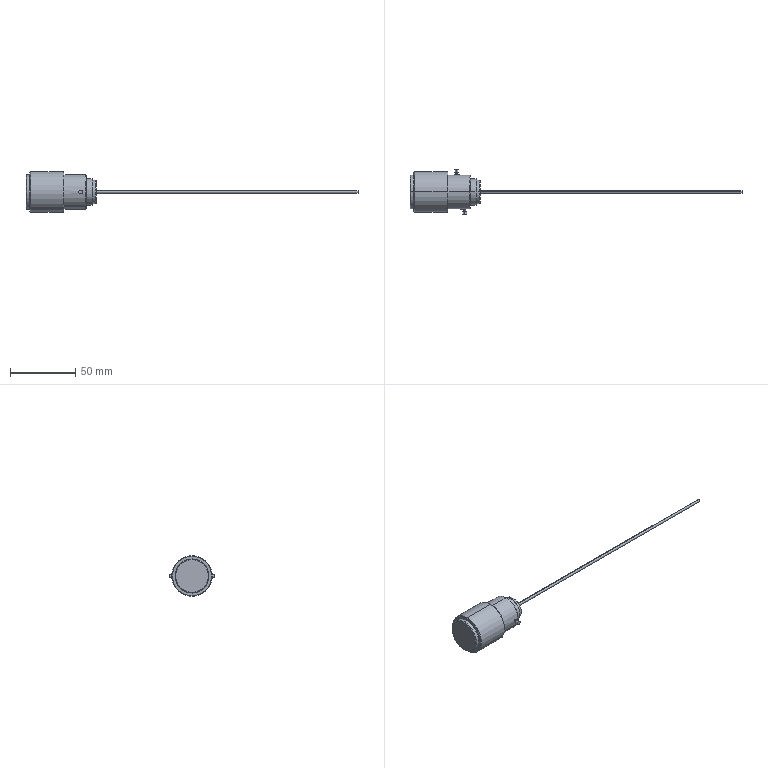Part | STEP file | Lens | 1 solid | 43 faces | box 253.5 x 35 x 31 mm | volume 33056 mm3 | cylinder 20 | cone 12 | plane 11 | commonest cylinder face diameters 26 x4 1.068 x2 1.193 x2 2 x2 2.761 x2 3 x2
STEP:
#1=CARTESIAN_POINT('',(-7.5,0.,-12.5));
#2=VERTEX_POINT('',#1);
#3=CARTESIAN_POINT('',(-7.5,0.,12.5));
#4=VERTEX_POINT('',#3);
#5=CARTESIAN_POINT('',(-7.5,0.,0.));
#6=DIRECTION('',(1.,0.,0.));
#7=DIRECTION('',(0.,0.,-1.));
#8=AXIS2_PLACEMENT_3D('',#5,#6,#7);
#9=CIRCLE('',#8,12.5);
#10=EDGE_CURVE('',#2,#4,#9,.T.);
#11=ORIENTED_EDGE('',*,*,#10,.F.);
#12=CARTESIAN_POINT('',(-8.,0.,-13.));
#13=VERTEX_POINT('',#12);
#14=CARTESIAN_POINT('',(-7.5,0.,-12.5));
#15=DIRECTION('',(-0.7071,0.,-0.7071));
#16=VECTOR('',#15,1000.);
#17=LINE('',#14,#16);
#18=EDGE_CURVE('',#2,#13,#17,.T.);
#19=ORIENTED_EDGE('',*,*,#18,.T.);
#20=CARTESIAN_POINT('',(-8.,0.,13.));
#21=VERTEX_POINT('',#20);
#22=CARTESIAN_POINT('',(-8.,0.,0.));
#23=DIRECTION('',(-1.,0.,0.));
#24=DIRECTION('',(0.,0.,-1.));
#25=AXIS2_PLACEMENT_3D('',#22,#23,#24);
#26=CIRCLE('',#25,13.);
#27=EDGE_CURVE('',#21,#13,#26,.T.);
#28=ORIENTED_EDGE('',*,*,#27,.F.);
#29=CARTESIAN_POINT('',(-7.5,0.,12.5));
#30=DIRECTION('',(-0.7071,0.,0.7071));
#31=VECTOR('',#30,1000.);
#32=LINE('',#29,#31);
#33=EDGE_CURVE('',#4,#21,#32,.T.);
#34=ORIENTED_EDGE('',*,*,#33,.F.);
#35=EDGE_LOOP('',(#11,#19,#28,#34));
#36=FACE_OUTER_BOUND('',#35,.T.);
#37=CARTESIAN_POINT('',(-7.5,0.,0.));
#38=DIRECTION('',(-1.,0.,0.));
#39=DIRECTION('',(0.,0.,1.));
#40=AXIS2_PLACEMENT_3D('',#37,#38,#39);
#41=CONICAL_SURFACE('',#40,12.5,0.7854);
#42=ADVANCED_FACE('',(#36),#41,.T.);
#43=CARTESIAN_POINT('',(0.,0.,-8.5));
#44=VERTEX_POINT('',#43);
#45=CARTESIAN_POINT('',(0.,0.,8.5));
#46=VERTEX_POINT('',#45);
#47=CARTESIAN_POINT('',(0.,0.,0.));
#48=DIRECTION('',(1.,0.,0.));
#49=DIRECTION('',(0.,0.,-1.));
#50=AXIS2_PLACEMENT_3D('',#47,#48,#49);
#51=CIRCLE('',#50,8.5);
#52=EDGE_CURVE('',#44,#46,#51,.T.);
#53=ORIENTED_EDGE('',*,*,#52,.F.);
#54=CARTESIAN_POINT('',(-0.5,0.,-9.));
#55=VERTEX_POINT('',#54);
#56=CARTESIAN_POINT('',(0.,0.,-8.5));
#57=DIRECTION('',(-0.7071,0.,-0.7071));
#58=VECTOR('',#57,1000.);
#59=LINE('',#56,#58);
#60=EDGE_CURVE('',#44,#55,#59,.T.);
#61=ORIENTED_EDGE('',*,*,#60,.T.);
#62=CARTESIAN_POINT('',(-0.5,0.,9.));
#63=VERTEX_POINT('',#62);
#64=CARTESIAN_POINT('',(-0.5,0.,0.));
#65=DIRECTION('',(-1.,0.,0.));
#66=DIRECTION('',(0.,0.,-1.));
#67=AXIS2_PLACEMENT_3D('',#64,#65,#66);
#68=CIRCLE('',#67,9.);
#69=EDGE_CURVE('',#63,#55,#68,.T.);
#70=ORIENTED_EDGE('',*,*,#69,.F.);
#71=CARTESIAN_POINT('',(0.,0.,8.5));
#72=DIRECTION('',(-0.7071,0.,0.7071));
#73=VECTOR('',#72,1000.);
#74=LINE('',#71,#73);
#75=EDGE_CURVE('',#46,#63,#74,.T.);
#76=ORIENTED_EDGE('',*,*,#75,.F.);
#77=EDGE_LOOP('',(#53,#61,#70,#76));
#78=FACE_OUTER_BOUND('',#77,.T.);
#79=CARTESIAN_POINT('',(0.,0.,0.));
#80=DIRECTION('',(-1.,0.,0.));
#81=DIRECTION('',(0.,0.,1.));
#82=AXIS2_PLACEMENT_3D('',#79,#80,#81);
#83=CONICAL_SURFACE('',#82,8.5,0.7854);
#84=ADVANCED_FACE('',(#78),#83,.T.);
#85=CARTESIAN_POINT('',(-2.5,0.,-9.5));
#86=VERTEX_POINT('',#85);
#87=CARTESIAN_POINT('',(-2.5,0.,9.5));
#88=VERTEX_POINT('',#87);
#89=CARTESIAN_POINT('',(-2.5,0.,0.));
#90=DIRECTION('',(1.,0.,0.));
#91=DIRECTION('',(0.,0.,-1.));
#92=AXIS2_PLACEMENT_3D('',#89,#90,#91);
#93=CIRCLE('',#92,9.5);
#94=EDGE_CURVE('',#86,#88,#93,.T.);
#95=ORIENTED_EDGE('',*,*,#94,.F.);
#96=CARTESIAN_POINT('',(-3.,0.,-10.));
#97=VERTEX_POINT('',#96);
#98=CARTESIAN_POINT('',(-2.5,0.,-9.5));
#99=DIRECTION('',(-0.7071,0.,-0.7071));
#100=VECTOR('',#99,1000.);
#101=LINE('',#98,#100);
#102=EDGE_CURVE('',#86,#97,#101,.T.);
#103=ORIENTED_EDGE('',*,*,#102,.T.);
#104=CARTESIAN_POINT('',(-3.,0.,10.));
#105=VERTEX_POINT('',#104);
#106=CARTESIAN_POINT('',(-3.,0.,0.));
#107=DIRECTION('',(-1.,0.,0.));
#108=DIRECTION('',(0.,0.,-1.));
#109=AXIS2_PLACEMENT_3D('',#106,#107,#108);
#110=CIRCLE('',#109,10.);
#111=EDGE_CURVE('',#105,#97,#110,.T.);
#112=ORIENTED_EDGE('',*,*,#111,.F.);
#113=CARTESIAN_POINT('',(-2.5,0.,9.5));
#114=DIRECTION('',(-0.7071,0.,0.7071));
#115=VECTOR('',#114,1000.);
#116=LINE('',#113,#115);
#117=EDGE_CURVE('',#88,#105,#116,.T.);
#118=ORIENTED_EDGE('',*,*,#117,.F.);
#119=EDGE_LOOP('',(#95,#103,#112,#118));
#120=FACE_OUTER_BOUND('',#119,.T.);
#121=CARTESIAN_POINT('',(-2.5,0.,0.));
#122=DIRECTION('',(-1.,0.,0.));
#123=DIRECTION('',(0.,0.,1.));
#124=AXIS2_PLACEMENT_3D('',#121,#122,#123);
#125=CONICAL_SURFACE('',#124,9.5,0.7854);
#126=ADVANCED_FACE('',(#120),#125,.T.);
#127=CARTESIAN_POINT('',(-24.5,0.,-15.));
#128=VERTEX_POINT('',#127);
#129=CARTESIAN_POINT('',(-24.5,0.,15.));
#130=VERTEX_POINT('',#129);
#131=CARTESIAN_POINT('',(-24.5,0.,0.));
#132=DIRECTION('',(1.,0.,0.));
#133=DIRECTION('',(0.,0.,-1.));
#134=AXIS2_PLACEMENT_3D('',#131,#132,#133);
#135=CIRCLE('',#134,15.);
#136=EDGE_CURVE('',#128,#130,#135,.T.);
#137=ORIENTED_EDGE('',*,*,#136,.F.);
#138=CARTESIAN_POINT('',(-25.,0.,-15.5));
#139=VERTEX_POINT('',#138);
#140=CARTESIAN_POINT('',(-24.5,0.,-15.));
#141=DIRECTION('',(-0.7071,0.,-0.7071));
#142=VECTOR('',#141,1000.);
#143=LINE('',#140,#142);
#144=EDGE_CURVE('',#128,#139,#143,.T.);
#145=ORIENTED_EDGE('',*,*,#144,.T.);
#146=CARTESIAN_POINT('',(-25.,0.,15.5));
#147=VERTEX_POINT('',#146);
#148=CARTESIAN_POINT('',(-25.,0.,0.));
#149=DIRECTION('',(-1.,0.,0.));
#150=DIRECTION('',(0.,0.,-1.));
#151=AXIS2_PLACEMENT_3D('',#148,#149,#150);
#152=CIRCLE('',#151,15.5);
#153=EDGE_CURVE('',#147,#139,#152,.T.);
#154=ORIENTED_EDGE('',*,*,#153,.F.);
#155=CARTESIAN_POINT('',(-24.5,0.,15.));
#156=DIRECTION('',(-0.7071,0.,0.7071));
#157=VECTOR('',#156,1000.);
#158=LINE('',#155,#157);
#159=EDGE_CURVE('',#130,#147,#158,.T.);
#160=ORIENTED_EDGE('',*,*,#159,.F.);
#161=EDGE_LOOP('',(#137,#145,#154,#160));
#162=FACE_OUTER_BOUND('',#161,.T.);
#163=CARTESIAN_POINT('',(-24.5,0.,0.));
#164=DIRECTION('',(-1.,0.,0.));
#165=DIRECTION('',(0.,0.,1.));
#166=AXIS2_PLACEMENT_3D('',#163,#164,#165);
#167=CONICAL_SURFACE('',#166,15.,0.7854);
#168=ADVANCED_FACE('',(#162),#167,.T.);
#169=CARTESIAN_POINT('',(-50.5,0.,15.));
#170=VERTEX_POINT('',#169);
#171=CARTESIAN_POINT('',(-50.5,0.,-15.));
#172=VERTEX_POINT('',#171);
#173=CARTESIAN_POINT('',(-50.5,0.,0.));
#174=DIRECTION('',(-1.,0.,0.));
#175=DIRECTION('',(0.,0.,1.));
#176=AXIS2_PLACEMENT_3D('',#173,#174,#175);
#177=CIRCLE('',#176,15.);
#178=EDGE_CURVE('',#170,#172,#177,.T.);
#179=ORIENTED_EDGE('',*,*,#178,.F.);
#180=CARTESIAN_POINT('',(-50.,0.,15.5));
#181=VERTEX_POINT('',#180);
#182=CARTESIAN_POINT('',(-50.,0.,15.5));
#183=DIRECTION('',(0.7071,0.,0.7071));
#184=VECTOR('',#183,1000.);
#185=LINE('',#182,#184);
#186=EDGE_CURVE('',#170,#181,#185,.T.);
#187=ORIENTED_EDGE('',*,*,#186,.T.);
#188=CARTESIAN_POINT('',(-50.,0.,-15.5));
#189=VERTEX_POINT('',#188);
#190=CARTESIAN_POINT('',(-50.,0.,0.));
#191=DIRECTION('',(1.,0.,0.));
#192=DIRECTION('',(0.,0.,1.));
#193=AXIS2_PLACEMENT_3D('',#190,#191,#192);
#194=CIRCLE('',#193,15.5);
#195=EDGE_CURVE('',#189,#181,#194,.T.);
#196=ORIENTED_EDGE('',*,*,#195,.F.);
#197=CARTESIAN_POINT('',(-50.,0.,-15.5));
#198=DIRECTION('',(0.7071,0.,-0.7071));
#199=VECTOR('',#198,1000.);
#200=LINE('',#197,#199);
#201=EDGE_CURVE('',#172,#189,#200,.T.);
#202=ORIENTED_EDGE('',*,*,#201,.F.);
#203=EDGE_LOOP('',(#179,#187,#196,#202));
#204=FACE_OUTER_BOUND('',#203,.T.);
#205=CARTESIAN_POINT('',(-50.,0.,0.));
#206=DIRECTION('',(1.,0.,0.));
#207=DIRECTION('',(0.,0.,-1.));
#208=AXIS2_PLACEMENT_3D('',#205,#206,#207);
#209=CONICAL_SURFACE('',#208,15.5,0.7854);
#210=ADVANCED_FACE('',(#204),#209,.T.);
#211=CARTESIAN_POINT('',(-53.5,0.,12.5));
#212=VERTEX_POINT('',#211);
#213=CARTESIAN_POINT('',(-53.5,0.,-12.5));
#214=VERTEX_POINT('',#213);
#215=CARTESIAN_POINT('',(-53.5,0.,0.));
#216=DIRECTION('',(-1.,0.,0.));
#217=DIRECTION('',(0.,0.,1.));
#218=AXIS2_PLACEMENT_3D('',#215,#216,#217);
#219=CIRCLE('',#218,12.5);
#220=EDGE_CURVE('',#212,#214,#219,.T.);
#221=ORIENTED_EDGE('',*,*,#220,.F.);
#222=CARTESIAN_POINT('',(-53.,0.,13.));
#223=VERTEX_POINT('',#222);
#224=CARTESIAN_POINT('',(-53.5,0.,12.5));
#225=DIRECTION('',(0.7071,0.,0.7071));
#226=VECTOR('',#225,1000.);
#227=LINE('',#224,#226);
#228=EDGE_CURVE('',#212,#223,#227,.T.);
#229=ORIENTED_EDGE('',*,*,#228,.T.);
#230=CARTESIAN_POINT('',(-53.,0.,-13.));
#231=VERTEX_POINT('',#230);
#232=CARTESIAN_POINT('',(-53.,0.,0.));
#233=DIRECTION('',(1.,0.,0.));
#234=DIRECTION('',(0.,0.,1.));
#235=AXIS2_PLACEMENT_3D('',#232,#233,#234);
#236=CIRCLE('',#235,13.);
#237=EDGE_CURVE('',#231,#223,#236,.T.);
#238=ORIENTED_EDGE('',*,*,#237,.F.);
#239=CARTESIAN_POINT('',(-53.5,0.,-12.5));
#240=DIRECTION('',(0.7071,0.,-0.7071));
#241=VECTOR('',#240,1000.);
#242=LINE('',#239,#241);
#243=EDGE_CURVE('',#214,#231,#242,.T.);
#244=ORIENTED_EDGE('',*,*,#243,.F.);
#245=EDGE_LOOP('',(#221,#229,#238,#244));
#246=FACE_OUTER_BOUND('',#245,.T.);
#247=CARTESIAN_POINT('',(-53.5,0.,0.));
#248=DIRECTION('',(1.,0.,0.));
#249=DIRECTION('',(0.,0.,-1.));
#250=AXIS2_PLACEMENT_3D('',#247,#248,#249);
#251=CONICAL_SURFACE('',#250,12.5,0.7854);
#252=ADVANCED_FACE('',(#246),#251,.T.);
#253=CARTESIAN_POINT('',(-18.,17.5,-1.38));
#254=VERTEX_POINT('',#253);
#255=CARTESIAN_POINT('',(-18.,17.5,1.38));
#256=VERTEX_POINT('',#255);
#257=CARTESIAN_POINT('',(-18.,17.5,0.));
#258=DIRECTION('',(0.,-1.,0.));
#259=DIRECTION('',(0.,0.,-1.));
#260=AXIS2_PLACEMENT_3D('',#257,#258,#259);
#261=CIRCLE('',#260,1.38);
#262=EDGE_CURVE('',#254,#256,#261,.T.);
#263=ORIENTED_EDGE('',*,*,#262,.T.);
#264=CARTESIAN_POINT('',(-18.,15.,1.38));
#265=VERTEX_POINT('',#264);
#266=CARTESIAN_POINT('',(-18.,17.5,1.38));
#267=DIRECTION('',(0.,-1.,0.));
#268=VECTOR('',#267,1000.);
#269=LINE('',#266,#268);
#270=EDGE_CURVE('',#256,#265,#269,.T.);
#271=ORIENTED_EDGE('',*,*,#270,.T.);
#272=CARTESIAN_POINT('',(-18.,15.,-1.38));
#273=VERTEX_POINT('',#272);
#274=CARTESIAN_POINT('',(-18.,15.,0.));
#275=DIRECTION('',(0.,-1.,0.));
#276=DIRECTION('',(0.,0.,-1.));
#277=AXIS2_PLACEMENT_3D('',#274,#275,#276);
#278=CIRCLE('',#277,1.38);
#279=EDGE_CURVE('',#273,#265,#278,.T.);
#280=ORIENTED_EDGE('',*,*,#279,.F.);
#281=CARTESIAN_POINT('',(-18.,17.5,-1.38));
#282=DIRECTION('',(0.,-1.,0.));
#283=VECTOR('',#282,1000.);
#284=LINE('',#281,#283);
#285=EDGE_CURVE('',#254,#273,#284,.T.);
#286=ORIENTED_EDGE('',*,*,#285,.F.);
#287=EDGE_LOOP('',(#263,#271,#280,#286));
#288=FACE_OUTER_BOUND('',#287,.T.);
#289=CARTESIAN_POINT('',(-18.,17.5,0.));
#290=DIRECTION('',(0.,-1.,0.));
#291=DIRECTION('',(0.,0.,-1.));
#292=AXIS2_PLACEMENT_3D('',#289,#290,#291);
#293=CYLINDRICAL_SURFACE('',#292,1.38);
#294=ADVANCED_FACE('',(#288),#293,.T.);
#295=CARTESIAN_POINT('',(-18.,15.,-0.5341));
#296=VERTEX_POINT('',#295);
#297=CARTESIAN_POINT('',(-18.,15.,0.5341));
#298=VERTEX_POINT('',#297);
#299=CARTESIAN_POINT('',(-18.,15.,0.));
#300=DIRECTION('',(0.,-1.,0.));
#301=DIRECTION('',(0.,0.,-1.));
#302=AXIS2_PLACEMENT_3D('',#299,#300,#301);
#303=CIRCLE('',#302,0.5341);
#304=EDGE_CURVE('',#296,#298,#303,.T.);
#305=ORIENTED_EDGE('',*,*,#304,.T.);
#306=CARTESIAN_POINT('',(-18.,12.989,0.5341));
#307=VERTEX_POINT('',#306);
#308=CARTESIAN_POINT('',(-18.,17.5,0.5341));
#309=DIRECTION('',(0.,-1.,0.));
#310=VECTOR('',#309,1000.);
#311=LINE('',#308,#310);
#312=EDGE_CURVE('',#298,#307,#311,.T.);
#313=ORIENTED_EDGE('',*,*,#312,.T.);
#314=CARTESIAN_POINT('',(-18.,12.989,-0.5341));
#315=VERTEX_POINT('',#314);
#316=CARTESIAN_POINT('',(-18.,12.989,-0.5341));
#317=CARTESIAN_POINT('',(-17.859,12.989,-0.5341));
#318=CARTESIAN_POINT('',(-17.721,12.992,-0.4762));
#319=CARTESIAN_POINT('',(-17.524,12.997,-0.279));
#320=CARTESIAN_POINT('',(-17.466,13.,-0.1395));
#321=CARTESIAN_POINT('',(-17.466,13.,0.1392));
#322=CARTESIAN_POINT('',(-17.523,12.997,0.2778));
#323=CARTESIAN_POINT('',(-17.722,12.992,0.4773));
#324=CARTESIAN_POINT('',(-17.861,12.989,0.5341));
#325=CARTESIAN_POINT('',(-18.,12.989,0.5341));
#326=B_SPLINE_CURVE_WITH_KNOTS('',3,(#316,#317,#318,#319,#320,#321,#322,#323,#324,#325),.UNSPECIFIED.,.F.,.F.,(4,2,2,2,4),(0.,0.0004175,0.000835,0.001252,0.00167),.UNSPECIFIED.);
#327=EDGE_CURVE('',#315,#307,#326,.T.);
#328=ORIENTED_EDGE('',*,*,#327,.F.);
#329=CARTESIAN_POINT('',(-18.,17.5,-0.5341));
#330=DIRECTION('',(0.,-1.,0.));
#331=VECTOR('',#330,1000.);
#332=LINE('',#329,#331);
#333=EDGE_CURVE('',#296,#315,#332,.T.);
#334=ORIENTED_EDGE('',*,*,#333,.F.);
#335=EDGE_LOOP('',(#305,#313,#328,#334));
#336=FACE_OUTER_BOUND('',#335,.T.);
#337=CARTESIAN_POINT('',(-18.,17.5,0.));
#338=DIRECTION('',(0.,-1.,0.));
#339=DIRECTION('',(0.,0.,-1.));
#340=AXIS2_PLACEMENT_3D('',#337,#338,#339);
#341=CYLINDRICAL_SURFACE('',#340,0.5341);
#342=ADVANCED_FACE('',(#336),#341,.T.);
#343=CARTESIAN_POINT('',(-11.694,-17.5,1.5));
#344=VERTEX_POINT('',#343);
#345=CARTESIAN_POINT('',(-11.694,-17.5,-1.5));
#346=VERTEX_POINT('',#345);
#347=CARTESIAN_POINT('',(-11.694,-17.5,0.));
#348=DIRECTION('',(0.,1.,0.));
#349=DIRECTION('',(0.,0.,1.));
#350=AXIS2_PLACEMENT_3D('',#347,#348,#349);
#351=CIRCLE('',#350,1.5);
#352=EDGE_CURVE('',#344,#346,#351,.T.);
#353=ORIENTED_EDGE('',*,*,#352,.T.);
#354=CARTESIAN_POINT('',(-11.694,-15.,-1.5));
#355=VERTEX_POINT('',#354);
#356=CARTESIAN_POINT('',(-11.694,-17.5,-1.5));
#357=DIRECTION('',(0.,1.,0.));
#358=VECTOR('',#357,1000.);
#359=LINE('',#356,#358);
#360=EDGE_CURVE('',#346,#355,#359,.T.);
#361=ORIENTED_EDGE('',*,*,#360,.T.);
#362=CARTESIAN_POINT('',(-11.694,-15.,1.5));
#363=VERTEX_POINT('',#362);
#364=CARTESIAN_POINT('',(-11.694,-15.,0.));
#365=DIRECTION('',(0.,1.,0.));
#366=DIRECTION('',(0.,0.,1.));
#367=AXIS2_PLACEMENT_3D('',#364,#365,#366);
#368=CIRCLE('',#367,1.5);
#369=EDGE_CURVE('',#363,#355,#368,.T.);
#370=ORIENTED_EDGE('',*,*,#369,.F.);
#371=CARTESIAN_POINT('',(-11.694,-17.5,1.5));
#372=DIRECTION('',(0.,1.,0.));
#373=VECTOR('',#372,1000.);
#374=LINE('',#371,#373);
#375=EDGE_CURVE('',#344,#363,#374,.T.);
#376=ORIENTED_EDGE('',*,*,#375,.F.);
#377=EDGE_LOOP('',(#353,#361,#370,#376));
#378=FACE_OUTER_BOUND('',#377,.T.);
#379=CARTESIAN_POINT('',(-11.694,-17.5,0.));
#380=DIRECTION('',(0.,1.,0.));
#381=DIRECTION('',(0.,0.,1.));
#382=AXIS2_PLACEMENT_3D('',#379,#380,#381);
#383=CYLINDRICAL_SURFACE('',#382,1.5);
#384=ADVANCED_FACE('',(#378),#383,.T.);
#385=CARTESIAN_POINT('',(-11.694,-15.,0.5963));
#386=VERTEX_POINT('',#385);
#387=CARTESIAN_POINT('',(-11.694,-15.,-0.5963));
#388=VERTEX_POINT('',#387);
#389=CARTESIAN_POINT('',(-11.694,-15.,0.));
#390=DIRECTION('',(0.,1.,0.));
#391=DIRECTION('',(0.,0.,1.));
#392=AXIS2_PLACEMENT_3D('',#389,#390,#391);
#393=CIRCLE('',#392,0.5963);
#394=EDGE_CURVE('',#386,#388,#393,.T.);
#395=ORIENTED_EDGE('',*,*,#394,.T.);
#396=CARTESIAN_POINT('',(-11.694,-12.986,-0.5963));
#397=VERTEX_POINT('',#396);
#398=CARTESIAN_POINT('',(-11.694,-17.5,-0.5963));
#399=DIRECTION('',(0.,1.,0.));
#400=VECTOR('',#399,1000.);
#401=LINE('',#398,#400);
#402=EDGE_CURVE('',#388,#397,#401,.T.);
#403=ORIENTED_EDGE('',*,*,#402,.T.);
#404=CARTESIAN_POINT('',(-11.694,-12.986,0.5963));
#405=VERTEX_POINT('',#404);
#406=CARTESIAN_POINT('',(-11.694,-12.986,0.5963));
#407=CARTESIAN_POINT('',(-11.536,-12.986,0.5963));
#408=CARTESIAN_POINT('',(-11.382,-12.99,0.5317));
#409=CARTESIAN_POINT('',(-11.162,-12.997,0.3116));
#410=CARTESIAN_POINT('',(-11.098,-13.,0.1558));
#411=CARTESIAN_POINT('',(-11.098,-13.,-0.1554));
#412=CARTESIAN_POINT('',(-11.161,-12.997,-0.3102));
#413=CARTESIAN_POINT('',(-11.384,-12.99,-0.533));
#414=CARTESIAN_POINT('',(-11.538,-12.986,-0.5963));
#415=CARTESIAN_POINT('',(-11.694,-12.986,-0.5963));
#416=B_SPLINE_CURVE_WITH_KNOTS('',3,(#406,#407,#408,#409,#410,#411,#412,#413,#414,#415),.UNSPECIFIED.,.F.,.F.,(4,2,2,2,4),(0.,0.0004662,0.0009323,0.001399,0.001865),.UNSPECIFIED.);
#417=EDGE_CURVE('',#405,#397,#416,.T.);
#418=ORIENTED_EDGE('',*,*,#417,.F.);
#419=CARTESIAN_POINT('',(-11.694,-17.5,0.5963));
#420=DIRECTION('',(0.,1.,0.));
#421=VECTOR('',#420,1000.);
#422=LINE('',#419,#421);
#423=EDGE_CURVE('',#386,#405,#422,.T.);
#424=ORIENTED_EDGE('',*,*,#423,.F.);
#425=EDGE_LOOP('',(#395,#403,#418,#424));
#426=FACE_OUTER_BOUND('',#425,.T.);
#427=CARTESIAN_POINT('',(-11.694,-17.5,0.));
#428=DIRECTION('',(0.,1.,0.));
#429=DIRECTION('',(0.,0.,1.));
#430=AXIS2_PLACEMENT_3D('',#427,#428,#429);
#431=CYLINDRICAL_SURFACE('',#430,0.5963);
#432=ADVANCED_FACE('',(#426),#431,.T.);
#433=ORIENTED_EDGE('',*,*,#237,.T.);
#434=CARTESIAN_POINT('',(-50.5,0.,13.));
#435=VERTEX_POINT('',#434);
#436=CARTESIAN_POINT('',(-53.5,0.,13.));
#437=DIRECTION('',(1.,0.,0.));
#438=VECTOR('',#437,1000.);
#439=LINE('',#436,#438);
#440=EDGE_CURVE('',#223,#435,#439,.T.);
#441=ORIENTED_EDGE('',*,*,#440,.T.);
#442=CARTESIAN_POINT('',(-50.5,0.,-13.));
#443=VERTEX_POINT('',#442);
#444=CARTESIAN_POINT('',(-50.5,0.,0.));
#445=DIRECTION('',(-1.,0.,0.));
#446=DIRECTION('',(0.,0.,1.));
#447=AXIS2_PLACEMENT_3D('',#444,#445,#446);
#448=CIRCLE('',#447,13.);
#449=EDGE_CURVE('',#435,#443,#448,.T.);
#450=ORIENTED_EDGE('',*,*,#449,.T.);
#451=CARTESIAN_POINT('',(-53.5,0.,-13.));
#452=DIRECTION('',(1.,0.,0.));
#453=VECTOR('',#452,1000.);
#454=LINE('',#451,#453);
#455=EDGE_CURVE('',#231,#443,#454,.T.);
#456=ORIENTED_EDGE('',*,*,#455,.F.);
#457=EDGE_LOOP('',(#433,#441,#450,#456));
#458=FACE_OUTER_BOUND('',#457,.T.);
#459=CARTESIAN_POINT('',(-53.5,0.,0.));
#460=DIRECTION('',(1.,0.,0.));
#461=DIRECTION('',(0.,0.,-1.));
#462=AXIS2_PLACEMENT_3D('',#459,#460,#461);
#463=CYLINDRICAL_SURFACE('',#462,13.);
#464=ADVANCED_FACE('',(#458),#463,.T.);
#465=ORIENTED_EDGE('',*,*,#69,.T.);
#466=CARTESIAN_POINT('',(-2.5,0.,-9.));
#467=VERTEX_POINT('',#466);
#468=CARTESIAN_POINT('',(0.,0.,-9.));
#469=DIRECTION('',(-1.,0.,0.));
#470=VECTOR('',#469,1000.);
#471=LINE('',#468,#470);
#472=EDGE_CURVE('',#55,#467,#471,.T.);
#473=ORIENTED_EDGE('',*,*,#472,.T.);
#474=CARTESIAN_POINT('',(-2.5,0.,9.));
#475=VERTEX_POINT('',#474);
#476=CARTESIAN_POINT('',(-2.5,0.,0.));
#477=DIRECTION('',(1.,0.,0.));
#478=DIRECTION('',(0.,0.,-1.));
#479=AXIS2_PLACEMENT_3D('',#476,#477,#478);
#480=CIRCLE('',#479,9.);
#481=EDGE_CURVE('',#467,#475,#480,.T.);
#482=ORIENTED_EDGE('',*,*,#481,.T.);
#483=CARTESIAN_POINT('',(0.,0.,9.));
#484=DIRECTION('',(-1.,0.,0.));
#485=VECTOR('',#484,1000.);
#486=LINE('',#483,#485);
#487=EDGE_CURVE('',#63,#475,#486,.T.);
#488=ORIENTED_EDGE('',*,*,#487,.F.);
#489=EDGE_LOOP('',(#465,#473,#482,#488));
#490=FACE_OUTER_BOUND('',#489,.T.);
#491=CARTESIAN_POINT('',(0.,0.,0.));
#492=DIRECTION('',(-1.,0.,0.));
#493=DIRECTION('',(0.,0.,1.));
#494=AXIS2_PLACEMENT_3D('',#491,#492,#493);
#495=CYLINDRICAL_SURFACE('',#494,9.);
#496=ADVANCED_FACE('',(#490),#495,.T.);
#497=ORIENTED_EDGE('',*,*,#111,.T.);
#498=CARTESIAN_POINT('',(-7.5,0.,-10.));
#499=VERTEX_POINT('',#498);
#500=CARTESIAN_POINT('',(-2.5,0.,-10.));
#501=DIRECTION('',(-1.,0.,0.));
#502=VECTOR('',#501,1000.);
#503=LINE('',#500,#502);
#504=EDGE_CURVE('',#97,#499,#503,.T.);
#505=ORIENTED_EDGE('',*,*,#504,.T.);
#506=CARTESIAN_POINT('',(-7.5,0.,10.));
#507=VERTEX_POINT('',#506);
#508=CARTESIAN_POINT('',(-7.5,0.,0.));
#509=DIRECTION('',(1.,0.,0.));
#510=DIRECTION('',(0.,0.,-1.));
#511=AXIS2_PLACEMENT_3D('',#508,#509,#510);
#512=CIRCLE('',#511,10.);
#513=EDGE_CURVE('',#499,#507,#512,.T.);
#514=ORIENTED_EDGE('',*,*,#513,.T.);
#515=CARTESIAN_POINT('',(-2.5,0.,10.));
#516=DIRECTION('',(-1.,0.,0.));
#517=VECTOR('',#516,1000.);
#518=LINE('',#515,#517);
#519=EDGE_CURVE('',#105,#507,#518,.T.);
#520=ORIENTED_EDGE('',*,*,#519,.F.);
#521=EDGE_LOOP('',(#497,#505,#514,#520));
#522=FACE_OUTER_BOUND('',#521,.T.);
#523=CARTESIAN_POINT('',(-2.5,0.,0.));
#524=DIRECTION('',(-1.,0.,0.));
#525=DIRECTION('',(0.,0.,1.));
#526=AXIS2_PLACEMENT_3D('',#523,#524,#525);
#527=CYLINDRICAL_SURFACE('',#526,10.);
#528=ADVANCED_FACE('',(#522),#527,.T.);
#529=ORIENTED_EDGE('',*,*,#327,.T.);
#530=CARTESIAN_POINT('',(-18.,12.989,0.5341));
#531=CARTESIAN_POINT('',(-18.139,12.989,0.5341));
#532=CARTESIAN_POINT('',(-18.279,12.992,0.4763));
#533=CARTESIAN_POINT('',(-18.476,12.997,0.2795));
#534=CARTESIAN_POINT('',(-18.534,13.,0.1413));
#535=CARTESIAN_POINT('',(-18.534,13.,-0.1405));
#536=CARTESIAN_POINT('',(-18.476,12.997,-0.2787));
#537=CARTESIAN_POINT('',(-18.279,12.992,-0.476));
#538=CARTESIAN_POINT('',(-18.141,12.989,-0.5341));
#539=CARTESIAN_POINT('',(-18.,12.989,-0.5341));
#540=B_SPLINE_CURVE_WITH_KNOTS('',3,(#530,#531,#532,#533,#534,#535,#536,#537,#538,#539),.UNSPECIFIED.,.F.,.F.,(4,2,2,2,4),(0.00167,0.002087,0.002505,0.002922,0.00334),.UNSPECIFIED.);
#541=EDGE_CURVE('',#307,#315,#540,.T.);
#542=ORIENTED_EDGE('',*,*,#541,.T.);
#543=EDGE_LOOP('',(#529,#542));
#544=FACE_BOUND('',#543,.T.);
#545=ORIENTED_EDGE('',*,*,#27,.T.);
#546=CARTESIAN_POINT('',(-24.5,0.,-13.));
#547=VERTEX_POINT('',#546);
#548=CARTESIAN_POINT('',(-7.5,0.,-13.));
#549=DIRECTION('',(-1.,0.,0.));
#550=VECTOR('',#549,1000.);
#551=LINE('',#548,#550);
#552=EDGE_CURVE('',#13,#547,#551,.T.);
#553=ORIENTED_EDGE('',*,*,#552,.T.);
#554=CARTESIAN_POINT('',(-24.5,0.,13.));
#555=VERTEX_POINT('',#554);
#556=CARTESIAN_POINT('',(-24.5,0.,0.));
#557=DIRECTION('',(1.,0.,0.));
#558=DIRECTION('',(0.,0.,-1.));
#559=AXIS2_PLACEMENT_3D('',#556,#557,#558);
#560=CIRCLE('',#559,13.);
#561=EDGE_CURVE('',#547,#555,#560,.T.);
#562=ORIENTED_EDGE('',*,*,#561,.T.);
#563=CARTESIAN_POINT('',(-7.5,0.,13.));
#564=DIRECTION('',(-1.,0.,0.));
#565=VECTOR('',#564,1000.);
#566=LINE('',#563,#565);
#567=EDGE_CURVE('',#21,#555,#566,.T.);
#568=ORIENTED_EDGE('',*,*,#567,.F.);
#569=EDGE_LOOP('',(#545,#553,#562,#568));
#570=FACE_OUTER_BOUND('',#569,.T.);
#571=CARTESIAN_POINT('',(-7.5,0.,0.));
#572=DIRECTION('',(-1.,0.,0.));
#573=DIRECTION('',(0.,0.,1.));
#574=AXIS2_PLACEMENT_3D('',#571,#572,#573);
#575=CYLINDRICAL_SURFACE('',#574,13.);
#576=ADVANCED_FACE('',(#544,#570),#575,.T.);
#577=ORIENTED_EDGE('',*,*,#195,.T.);
#578=CARTESIAN_POINT('',(-50.5,0.,15.5));
#579=DIRECTION('',(1.,0.,0.));
#580=VECTOR('',#579,1000.);
#581=LINE('',#578,#580);
#582=EDGE_CURVE('',#181,#147,#581,.T.);
#583=ORIENTED_EDGE('',*,*,#582,.T.);
#584=ORIENTED_EDGE('',*,*,#153,.T.);
#585=CARTESIAN_POINT('',(-50.5,0.,-15.5));
#586=DIRECTION('',(1.,0.,0.));
#587=VECTOR('',#586,1000.);
#588=LINE('',#585,#587);
#589=EDGE_CURVE('',#189,#139,#588,.T.);
#590=ORIENTED_EDGE('',*,*,#589,.F.);
#591=EDGE_LOOP('',(#577,#583,#584,#590));
#592=FACE_OUTER_BOUND('',#591,.T.);
#593=CARTESIAN_POINT('',(-50.5,0.,0.));
#594=DIRECTION('',(1.,0.,0.));
#595=DIRECTION('',(0.,0.,-1.));
#596=AXIS2_PLACEMENT_3D('',#593,#594,#595);
#597=CYLINDRICAL_SURFACE('',#596,15.5);
#598=ADVANCED_FACE('',(#592),#597,.T.);
#599=CARTESIAN_POINT('',(200.,0.,-1.));
#600=VERTEX_POINT('',#599);
#601=CARTESIAN_POINT('',(200.,0.,1.));
#602=VERTEX_POINT('',#601);
#603=CARTESIAN_POINT('',(200.,0.,0.));
#604=DIRECTION('',(1.,0.,0.));
#605=DIRECTION('',(0.,0.,-1.));
#606=AXIS2_PLACEMENT_3D('',#603,#604,#605);
#607=CIRCLE('',#606,1.);
#608=EDGE_CURVE('',#600,#602,#607,.T.);
#609=ORIENTED_EDGE('',*,*,#608,.F.);
#610=CARTESIAN_POINT('',(0.,0.,-1.));
#611=VERTEX_POINT('',#610);
#612=CARTESIAN_POINT('',(280.,0.,-1.));
#613=DIRECTION('',(-1.,0.,0.));
#614=VECTOR('',#613,1000.);
#615=LINE('',#612,#614);
#616=EDGE_CURVE('',#600,#611,#615,.T.);
#617=ORIENTED_EDGE('',*,*,#616,.T.);
#618=CARTESIAN_POINT('',(0.,0.,1.));
#619=VERTEX_POINT('',#618);
#620=CARTESIAN_POINT('',(0.,0.,0.));
#621=DIRECTION('',(1.,0.,0.));
#622=DIRECTION('',(0.,0.,-1.));
#623=AXIS2_PLACEMENT_3D('',#620,#621,#622);
#624=CIRCLE('',#623,1.);
#625=EDGE_CURVE('',#611,#619,#624,.T.);
#626=ORIENTED_EDGE('',*,*,#625,.T.);
#627=CARTESIAN_POINT('',(280.,0.,1.));
#628=DIRECTION('',(-1.,0.,0.));
#629=VECTOR('',#628,1000.);
#630=LINE('',#627,#629);
#631=EDGE_CURVE('',#602,#619,#630,.T.);
#632=ORIENTED_EDGE('',*,*,#631,.F.);
#633=EDGE_LOOP('',(#609,#617,#626,#632));
#634=FACE_OUTER_BOUND('',#633,.T.);
#635=CARTESIAN_POINT('',(280.,0.,0.));
#636=DIRECTION('',(-1.,0.,0.));
#637=DIRECTION('',(0.,0.,1.));
#638=AXIS2_PLACEMENT_3D('',#635,#636,#637);
#639=CYLINDRICAL_SURFACE('',#638,1.);
#640=ADVANCED_FACE('',(#634),#639,.T.);
#641=ORIENTED_EDGE('',*,*,#616,.F.);
#642=CARTESIAN_POINT('',(200.,0.,0.));
#643=DIRECTION('',(1.,0.,0.));
#644=DIRECTION('',(0.,0.,-1.));
#645=AXIS2_PLACEMENT_3D('',#642,#643,#644);
#646=CIRCLE('',#645,1.);
#647=EDGE_CURVE('',#602,#600,#646,.T.);
#648=ORIENTED_EDGE('',*,*,#647,.F.);
#649=ORIENTED_EDGE('',*,*,#631,.T.);
#650=CARTESIAN_POINT('',(0.,0.,0.));
#651=DIRECTION('',(1.,0.,0.));
#652=DIRECTION('',(0.,0.,-1.));
#653=AXIS2_PLACEMENT_3D('',#650,#651,#652);
#654=CIRCLE('',#653,1.);
#655=EDGE_CURVE('',#619,#611,#654,.T.);
#656=ORIENTED_EDGE('',*,*,#655,.T.);
#657=EDGE_LOOP('',(#641,#648,#649,#656));
#658=FACE_OUTER_BOUND('',#657,.T.);
#659=CARTESIAN_POINT('',(280.,0.,0.));
#660=DIRECTION('',(-1.,0.,0.));
#661=DIRECTION('',(0.,0.,1.));
#662=AXIS2_PLACEMENT_3D('',#659,#660,#661);
#663=CYLINDRICAL_SURFACE('',#662,1.);
#664=ADVANCED_FACE('',(#658),#663,.T.);
#665=CARTESIAN_POINT('',(-50.5,0.,0.));
#666=DIRECTION('',(-1.,0.,0.));
#667=DIRECTION('',(0.,0.,1.));
#668=AXIS2_PLACEMENT_3D('',#665,#666,#667);
#669=CIRCLE('',#668,15.);
#670=EDGE_CURVE('',#172,#170,#669,.T.);
#671=ORIENTED_EDGE('',*,*,#670,.T.);
#672=ORIENTED_EDGE('',*,*,#178,.T.);
#673=EDGE_LOOP('',(#671,#672));
#674=FACE_OUTER_BOUND('',#673,.T.);
#675=CARTESIAN_POINT('',(-50.5,0.,0.));
#676=DIRECTION('',(-1.,0.,0.));
#677=DIRECTION('',(0.,0.,1.));
#678=AXIS2_PLACEMENT_3D('',#675,#676,#677);
#679=CIRCLE('',#678,13.);
#680=EDGE_CURVE('',#443,#435,#679,.T.);
#681=ORIENTED_EDGE('',*,*,#680,.F.);
#682=ORIENTED_EDGE('',*,*,#449,.F.);
#683=EDGE_LOOP('',(#681,#682));
#684=FACE_BOUND('',#683,.T.);
#685=CARTESIAN_POINT('',(-50.5,15.5,0.));
#686=DIRECTION('',(-1.,0.,0.));
#687=DIRECTION('',(0.,0.,1.));
#688=AXIS2_PLACEMENT_3D('',#685,#686,#687);
#689=PLANE('',#688);
#690=ADVANCED_FACE('',(#674,#684),#689,.T.);
#691=CARTESIAN_POINT('',(0.,0.,0.));
#692=DIRECTION('',(1.,0.,0.));
#693=DIRECTION('',(0.,0.,-1.));
#694=AXIS2_PLACEMENT_3D('',#691,#692,#693);
#695=CIRCLE('',#694,8.5);
#696=EDGE_CURVE('',#46,#44,#695,.T.);
#697=ORIENTED_EDGE('',*,*,#696,.T.);
#698=ORIENTED_EDGE('',*,*,#52,.T.);
#699=EDGE_LOOP('',(#697,#698));
#700=FACE_OUTER_BOUND('',#699,.T.);
#701=ORIENTED_EDGE('',*,*,#655,.F.);
#702=ORIENTED_EDGE('',*,*,#625,.F.);
#703=EDGE_LOOP('',(#701,#702));
#704=FACE_BOUND('',#703,.T.);
#705=CARTESIAN_POINT('',(0.,0.,0.));
#706=DIRECTION('',(1.,0.,0.));
#707=DIRECTION('',(0.,0.,-1.));
#708=AXIS2_PLACEMENT_3D('',#705,#706,#707);
#709=PLANE('',#708);
#710=ADVANCED_FACE('',(#700,#704),#709,.T.);
#711=CARTESIAN_POINT('',(-2.5,0.,0.));
#712=DIRECTION('',(1.,0.,0.));
#713=DIRECTION('',(0.,0.,-1.));
#714=AXIS2_PLACEMENT_3D('',#711,#712,#713);
#715=CIRCLE('',#714,9.5);
#716=EDGE_CURVE('',#88,#86,#715,.T.);
#717=ORIENTED_EDGE('',*,*,#716,.T.);
#718=ORIENTED_EDGE('',*,*,#94,.T.);
#719=EDGE_LOOP('',(#717,#718));
#720=FACE_OUTER_BOUND('',#719,.T.);
#721=CARTESIAN_POINT('',(-2.5,0.,0.));
#722=DIRECTION('',(1.,0.,0.));
#723=DIRECTION('',(0.,0.,-1.));
#724=AXIS2_PLACEMENT_3D('',#721,#722,#723);
#725=CIRCLE('',#724,9.);
#726=EDGE_CURVE('',#475,#467,#725,.T.);
#727=ORIENTED_EDGE('',*,*,#726,.F.);
#728=ORIENTED_EDGE('',*,*,#481,.F.);
#729=EDGE_LOOP('',(#727,#728));
#730=FACE_BOUND('',#729,.T.);
#731=CARTESIAN_POINT('',(-2.5,0.,0.));
#732=DIRECTION('',(1.,0.,0.));
#733=DIRECTION('',(0.,0.,-1.));
#734=AXIS2_PLACEMENT_3D('',#731,#732,#733);
#735=PLANE('',#734);
#736=ADVANCED_FACE('',(#720,#730),#735,.T.);
#737=CARTESIAN_POINT('',(-7.5,0.,0.));
#738=DIRECTION('',(1.,0.,0.));
#739=DIRECTION('',(0.,0.,-1.));
#740=AXIS2_PLACEMENT_3D('',#737,#738,#739);
#741=CIRCLE('',#740,12.5);
#742=EDGE_CURVE('',#4,#2,#741,.T.);
#743=ORIENTED_EDGE('',*,*,#742,.T.);
#744=ORIENTED_EDGE('',*,*,#10,.T.);
#745=EDGE_LOOP('',(#743,#744));
#746=FACE_OUTER_BOUND('',#745,.T.);
#747=CARTESIAN_POINT('',(-7.5,0.,0.));
#748=DIRECTION('',(1.,0.,0.));
#749=DIRECTION('',(0.,0.,-1.));
#750=AXIS2_PLACEMENT_3D('',#747,#748,#749);
#751=CIRCLE('',#750,10.);
#752=EDGE_CURVE('',#507,#499,#751,.T.);
#753=ORIENTED_EDGE('',*,*,#752,.F.);
#754=ORIENTED_EDGE('',*,*,#513,.F.);
#755=EDGE_LOOP('',(#753,#754));
#756=FACE_BOUND('',#755,.T.);
#757=CARTESIAN_POINT('',(-7.5,0.,0.));
#758=DIRECTION('',(1.,0.,0.));
#759=DIRECTION('',(0.,0.,-1.));
#760=AXIS2_PLACEMENT_3D('',#757,#758,#759);
#761=PLANE('',#760);
#762=ADVANCED_FACE('',(#746,#756),#761,.T.);
#763=CARTESIAN_POINT('',(-24.5,0.,0.));
#764=DIRECTION('',(1.,0.,0.));
#765=DIRECTION('',(0.,0.,-1.));
#766=AXIS2_PLACEMENT_3D('',#763,#764,#765);
#767=CIRCLE('',#766,15.);
#768=EDGE_CURVE('',#130,#128,#767,.T.);
#769=ORIENTED_EDGE('',*,*,#768,.T.);
#770=ORIENTED_EDGE('',*,*,#136,.T.);
#771=EDGE_LOOP('',(#769,#770));
#772=FACE_OUTER_BOUND('',#771,.T.);
#773=CARTESIAN_POINT('',(-24.5,0.,0.));
#774=DIRECTION('',(1.,0.,0.));
#775=DIRECTION('',(0.,0.,-1.));
#776=AXIS2_PLACEMENT_3D('',#773,#774,#775);
#777=CIRCLE('',#776,13.);
#778=EDGE_CURVE('',#555,#547,#777,.T.);
#779=ORIENTED_EDGE('',*,*,#778,.F.);
#780=ORIENTED_EDGE('',*,*,#561,.F.);
#781=EDGE_LOOP('',(#779,#780));
#782=FACE_BOUND('',#781,.T.);
#783=CARTESIAN_POINT('',(-24.5,0.,0.));
#784=DIRECTION('',(1.,0.,0.));
#785=DIRECTION('',(0.,0.,-1.));
#786=AXIS2_PLACEMENT_3D('',#783,#784,#785);
#787=PLANE('',#786);
#788=ADVANCED_FACE('',(#772,#782),#787,.T.);
#789=ORIENTED_EDGE('',*,*,#582,.F.);
#790=CARTESIAN_POINT('',(-50.,0.,0.));
#791=DIRECTION('',(1.,0.,0.));
#792=DIRECTION('',(0.,0.,1.));
#793=AXIS2_PLACEMENT_3D('',#790,#791,#792);
#794=CIRCLE('',#793,15.5);
#795=EDGE_CURVE('',#181,#189,#794,.T.);
#796=ORIENTED_EDGE('',*,*,#795,.T.);
#797=ORIENTED_EDGE('',*,*,#589,.T.);
#798=CARTESIAN_POINT('',(-25.,0.,0.));
#799=DIRECTION('',(-1.,0.,0.));
#800=DIRECTION('',(0.,0.,-1.));
#801=AXIS2_PLACEMENT_3D('',#798,#799,#800);
#802=CIRCLE('',#801,15.5);
#803=EDGE_CURVE('',#139,#147,#802,.T.);
#804=ORIENTED_EDGE('',*,*,#803,.T.);
#805=EDGE_LOOP('',(#789,#796,#797,#804));
#806=FACE_OUTER_BOUND('',#805,.T.);
#807=CARTESIAN_POINT('',(-50.5,0.,0.));
#808=DIRECTION('',(1.,0.,0.));
#809=DIRECTION('',(0.,0.,-1.));
#810=AXIS2_PLACEMENT_3D('',#807,#808,#809);
#811=CYLINDRICAL_SURFACE('',#810,15.5);
#812=ADVANCED_FACE('',(#806),#811,.T.);
#813=ORIENTED_EDGE('',*,*,#552,.F.);
#814=CARTESIAN_POINT('',(-8.,0.,0.));
#815=DIRECTION('',(-1.,0.,0.));
#816=DIRECTION('',(0.,0.,-1.));
#817=AXIS2_PLACEMENT_3D('',#814,#815,#816);
#818=CIRCLE('',#817,13.);
#819=EDGE_CURVE('',#13,#21,#818,.T.);
#820=ORIENTED_EDGE('',*,*,#819,.T.);
#821=ORIENTED_EDGE('',*,*,#567,.T.);
#822=ORIENTED_EDGE('',*,*,#778,.T.);
#823=EDGE_LOOP('',(#813,#820,#821,#822));
#824=FACE_OUTER_BOUND('',#823,.T.);
#825=ORIENTED_EDGE('',*,*,#417,.T.);
#826=CARTESIAN_POINT('',(-11.694,-12.986,-0.5963));
#827=CARTESIAN_POINT('',(-11.85,-12.986,-0.5963));
#828=CARTESIAN_POINT('',(-12.005,-12.99,-0.5319));
#829=CARTESIAN_POINT('',(-12.225,-12.997,-0.3121));
#830=CARTESIAN_POINT('',(-12.29,-13.,-0.1578));
#831=CARTESIAN_POINT('',(-12.29,-13.,0.1568));
#832=CARTESIAN_POINT('',(-12.226,-12.997,0.3112));
#833=CARTESIAN_POINT('',(-12.006,-12.99,0.5315));
#834=CARTESIAN_POINT('',(-11.852,-12.986,0.5963));
#835=CARTESIAN_POINT('',(-11.694,-12.986,0.5963));
#836=B_SPLINE_CURVE_WITH_KNOTS('',3,(#826,#827,#828,#829,#830,#831,#832,#833,#834,#835),.UNSPECIFIED.,.F.,.F.,(4,2,2,2,4),(0.001865,0.002331,0.002797,0.003263,0.003729),.UNSPECIFIED.);
#837=EDGE_CURVE('',#397,#405,#836,.T.);
#838=ORIENTED_EDGE('',*,*,#837,.T.);
#839=EDGE_LOOP('',(#825,#838));
#840=FACE_BOUND('',#839,.T.);
#841=CARTESIAN_POINT('',(-7.5,0.,0.));
#842=DIRECTION('',(-1.,0.,0.));
#843=DIRECTION('',(0.,0.,1.));
#844=AXIS2_PLACEMENT_3D('',#841,#842,#843);
#845=CYLINDRICAL_SURFACE('',#844,13.);
#846=ADVANCED_FACE('',(#824,#840),#845,.T.);
#847=ORIENTED_EDGE('',*,*,#504,.F.);
#848=CARTESIAN_POINT('',(-3.,0.,0.));
#849=DIRECTION('',(-1.,0.,0.));
#850=DIRECTION('',(0.,0.,-1.));
#851=AXIS2_PLACEMENT_3D('',#848,#849,#850);
#852=CIRCLE('',#851,10.);
#853=EDGE_CURVE('',#97,#105,#852,.T.);
#854=ORIENTED_EDGE('',*,*,#853,.T.);
#855=ORIENTED_EDGE('',*,*,#519,.T.);
#856=ORIENTED_EDGE('',*,*,#752,.T.);
#857=EDGE_LOOP('',(#847,#854,#855,#856));
#858=FACE_OUTER_BOUND('',#857,.T.);
#859=CARTESIAN_POINT('',(-2.5,0.,0.));
#860=DIRECTION('',(-1.,0.,0.));
#861=DIRECTION('',(0.,0.,1.));
#862=AXIS2_PLACEMENT_3D('',#859,#860,#861);
#863=CYLINDRICAL_SURFACE('',#862,10.);
#864=ADVANCED_FACE('',(#858),#863,.T.);
#865=ORIENTED_EDGE('',*,*,#472,.F.);
#866=CARTESIAN_POINT('',(-0.5,0.,0.));
#867=DIRECTION('',(-1.,0.,0.));
#868=DIRECTION('',(0.,0.,-1.));
#869=AXIS2_PLACEMENT_3D('',#866,#867,#868);
#870=CIRCLE('',#869,9.);
#871=EDGE_CURVE('',#55,#63,#870,.T.);
#872=ORIENTED_EDGE('',*,*,#871,.T.);
#873=ORIENTED_EDGE('',*,*,#487,.T.);
#874=ORIENTED_EDGE('',*,*,#726,.T.);
#875=EDGE_LOOP('',(#865,#872,#873,#874));
#876=FACE_OUTER_BOUND('',#875,.T.);
#877=CARTESIAN_POINT('',(0.,0.,0.));
#878=DIRECTION('',(-1.,0.,0.));
#879=DIRECTION('',(0.,0.,1.));
#880=AXIS2_PLACEMENT_3D('',#877,#878,#879);
#881=CYLINDRICAL_SURFACE('',#880,9.);
#882=ADVANCED_FACE('',(#876),#881,.T.);
#883=ORIENTED_EDGE('',*,*,#440,.F.);
#884=CARTESIAN_POINT('',(-53.,0.,0.));
#885=DIRECTION('',(1.,0.,0.));
#886=DIRECTION('',(0.,0.,1.));
#887=AXIS2_PLACEMENT_3D('',#884,#885,#886);
#888=CIRCLE('',#887,13.);
#889=EDGE_CURVE('',#223,#231,#888,.T.);
#890=ORIENTED_EDGE('',*,*,#889,.T.);
#891=ORIENTED_EDGE('',*,*,#455,.T.);
#892=ORIENTED_EDGE('',*,*,#680,.T.);
#893=EDGE_LOOP('',(#883,#890,#891,#892));
#894=FACE_OUTER_BOUND('',#893,.T.);
#895=CARTESIAN_POINT('',(-53.5,0.,0.));
#896=DIRECTION('',(1.,0.,0.));
#897=DIRECTION('',(0.,0.,-1.));
#898=AXIS2_PLACEMENT_3D('',#895,#896,#897);
#899=CYLINDRICAL_SURFACE('',#898,13.);
#900=ADVANCED_FACE('',(#894),#899,.T.);
#901=CARTESIAN_POINT('',(-53.5,0.,0.));
#902=DIRECTION('',(-1.,0.,0.));
#903=DIRECTION('',(0.,0.,1.));
#904=AXIS2_PLACEMENT_3D('',#901,#902,#903);
#905=CIRCLE('',#904,12.5);
#906=EDGE_CURVE('',#214,#212,#905,.T.);
#907=ORIENTED_EDGE('',*,*,#906,.T.);
#908=ORIENTED_EDGE('',*,*,#220,.T.);
#909=EDGE_LOOP('',(#907,#908));
#910=FACE_OUTER_BOUND('',#909,.T.);
#911=CARTESIAN_POINT('',(-53.5,0.,0.));
#912=DIRECTION('',(-1.,0.,0.));
#913=DIRECTION('',(0.,0.,1.));
#914=AXIS2_PLACEMENT_3D('',#911,#912,#913);
#915=PLANE('',#914);
#916=ADVANCED_FACE('',(#910),#915,.T.);
#917=ORIENTED_EDGE('',*,*,#402,.F.);
#918=CARTESIAN_POINT('',(-11.694,-15.,0.));
#919=DIRECTION('',(0.,1.,0.));
#920=DIRECTION('',(0.,0.,1.));
#921=AXIS2_PLACEMENT_3D('',#918,#919,#920);
#922=CIRCLE('',#921,0.5963);
#923=EDGE_CURVE('',#388,#386,#922,.T.);
#924=ORIENTED_EDGE('',*,*,#923,.T.);
#925=ORIENTED_EDGE('',*,*,#423,.T.);
#926=ORIENTED_EDGE('',*,*,#837,.F.);
#927=EDGE_LOOP('',(#917,#924,#925,#926));
#928=FACE_OUTER_BOUND('',#927,.T.);
#929=CARTESIAN_POINT('',(-11.694,-17.5,0.));
#930=DIRECTION('',(0.,1.,0.));
#931=DIRECTION('',(0.,0.,1.));
#932=AXIS2_PLACEMENT_3D('',#929,#930,#931);
#933=CYLINDRICAL_SURFACE('',#932,0.5963);
#934=ADVANCED_FACE('',(#928),#933,.T.);
#935=ORIENTED_EDGE('',*,*,#360,.F.);
#936=CARTESIAN_POINT('',(-11.694,-17.5,0.));
#937=DIRECTION('',(0.,1.,0.));
#938=DIRECTION('',(0.,0.,1.));
#939=AXIS2_PLACEMENT_3D('',#936,#937,#938);
#940=CIRCLE('',#939,1.5);
#941=EDGE_CURVE('',#346,#344,#940,.T.);
#942=ORIENTED_EDGE('',*,*,#941,.T.);
#943=ORIENTED_EDGE('',*,*,#375,.T.);
#944=CARTESIAN_POINT('',(-11.694,-15.,0.));
#945=DIRECTION('',(0.,1.,0.));
#946=DIRECTION('',(0.,0.,1.));
#947=AXIS2_PLACEMENT_3D('',#944,#945,#946);
#948=CIRCLE('',#947,1.5);
#949=EDGE_CURVE('',#355,#363,#948,.T.);
#950=ORIENTED_EDGE('',*,*,#949,.F.);
#951=EDGE_LOOP('',(#935,#942,#943,#950));
#952=FACE_OUTER_BOUND('',#951,.T.);
#953=CARTESIAN_POINT('',(-11.694,-17.5,0.));
#954=DIRECTION('',(0.,1.,0.));
#955=DIRECTION('',(0.,0.,1.));
#956=AXIS2_PLACEMENT_3D('',#953,#954,#955);
#957=CYLINDRICAL_SURFACE('',#956,1.5);
#958=ADVANCED_FACE('',(#952),#957,.T.);
#959=ORIENTED_EDGE('',*,*,#352,.F.);
#960=ORIENTED_EDGE('',*,*,#941,.F.);
#961=EDGE_LOOP('',(#959,#960));
#962=FACE_OUTER_BOUND('',#961,.T.);
#963=CARTESIAN_POINT('',(-11.694,-17.5,1.5));
#964=DIRECTION('',(0.,-1.,0.));
#965=DIRECTION('',(0.,0.,-1.));
#966=AXIS2_PLACEMENT_3D('',#963,#964,#965);
#967=PLANE('',#966);
#968=ADVANCED_FACE('',(#962),#967,.T.);
#969=ORIENTED_EDGE('',*,*,#369,.T.);
#970=ORIENTED_EDGE('',*,*,#949,.T.);
#971=EDGE_LOOP('',(#969,#970));
#972=FACE_OUTER_BOUND('',#971,.T.);
#973=ORIENTED_EDGE('',*,*,#394,.F.);
#974=ORIENTED_EDGE('',*,*,#923,.F.);
#975=EDGE_LOOP('',(#973,#974));
#976=FACE_BOUND('',#975,.T.);
#977=CARTESIAN_POINT('',(-11.694,-15.,0.5963));
#978=DIRECTION('',(0.,1.,0.));
#979=DIRECTION('',(0.,0.,1.));
#980=AXIS2_PLACEMENT_3D('',#977,#978,#979);
#981=PLANE('',#980);
#982=ADVANCED_FACE('',(#972,#976),#981,.T.);
#983=ORIENTED_EDGE('',*,*,#312,.F.);
#984=CARTESIAN_POINT('',(-18.,15.,0.));
#985=DIRECTION('',(0.,-1.,0.));
#986=DIRECTION('',(0.,0.,-1.));
#987=AXIS2_PLACEMENT_3D('',#984,#985,#986);
#988=CIRCLE('',#987,0.5341);
#989=EDGE_CURVE('',#298,#296,#988,.T.);
#990=ORIENTED_EDGE('',*,*,#989,.T.);
#991=ORIENTED_EDGE('',*,*,#333,.T.);
#992=ORIENTED_EDGE('',*,*,#541,.F.);
#993=EDGE_LOOP('',(#983,#990,#991,#992));
#994=FACE_OUTER_BOUND('',#993,.T.);
#995=CARTESIAN_POINT('',(-18.,17.5,0.));
#996=DIRECTION('',(0.,-1.,0.));
#997=DIRECTION('',(0.,0.,-1.));
#998=AXIS2_PLACEMENT_3D('',#995,#996,#997);
#999=CYLINDRICAL_SURFACE('',#998,0.5341);
#1000=ADVANCED_FACE('',(#994),#999,.T.);
#1001=ORIENTED_EDGE('',*,*,#270,.F.);
#1002=CARTESIAN_POINT('',(-18.,17.5,0.));
#1003=DIRECTION('',(0.,-1.,0.));
#1004=DIRECTION('',(0.,0.,-1.));
#1005=AXIS2_PLACEMENT_3D('',#1002,#1003,#1004);
#1006=CIRCLE('',#1005,1.38);
#1007=EDGE_CURVE('',#256,#254,#1006,.T.);
#1008=ORIENTED_EDGE('',*,*,#1007,.T.);
#1009=ORIENTED_EDGE('',*,*,#285,.T.);
#1010=CARTESIAN_POINT('',(-18.,15.,0.));
#1011=DIRECTION('',(0.,-1.,0.));
#1012=DIRECTION('',(0.,0.,-1.));
#1013=AXIS2_PLACEMENT_3D('',#1010,#1011,#1012);
#1014=CIRCLE('',#1013,1.38);
#1015=EDGE_CURVE('',#265,#273,#1014,.T.);
#1016=ORIENTED_EDGE('',*,*,#1015,.F.);
#1017=EDGE_LOOP('',(#1001,#1008,#1009,#1016));
#1018=FACE_OUTER_BOUND('',#1017,.T.);
#1019=CARTESIAN_POINT('',(-18.,17.5,0.));
#1020=DIRECTION('',(0.,-1.,0.));
#1021=DIRECTION('',(0.,0.,-1.));
#1022=AXIS2_PLACEMENT_3D('',#1019,#1020,#1021);
#1023=CYLINDRICAL_SURFACE('',#1022,1.38);
#1024=ADVANCED_FACE('',(#1018),#1023,.T.);
#1025=ORIENTED_EDGE('',*,*,#262,.F.);
#1026=ORIENTED_EDGE('',*,*,#1007,.F.);
#1027=EDGE_LOOP('',(#1025,#1026));
#1028=FACE_OUTER_BOUND('',#1027,.T.);
#1029=CARTESIAN_POINT('',(-18.,17.5,-1.38));
#1030=DIRECTION('',(0.,1.,0.));
#1031=DIRECTION('',(0.,0.,1.));
#1032=AXIS2_PLACEMENT_3D('',#1029,#1030,#1031);
#1033=PLANE('',#1032);
#1034=ADVANCED_FACE('',(#1028),#1033,.T.);
#1035=ORIENTED_EDGE('',*,*,#279,.T.);
#1036=ORIENTED_EDGE('',*,*,#1015,.T.);
#1037=EDGE_LOOP('',(#1035,#1036));
#1038=FACE_OUTER_BOUND('',#1037,.T.);
#1039=ORIENTED_EDGE('',*,*,#304,.F.);
#1040=ORIENTED_EDGE('',*,*,#989,.F.);
#1041=EDGE_LOOP('',(#1039,#1040));
#1042=FACE_BOUND('',#1041,.T.);
#1043=CARTESIAN_POINT('',(-18.,15.,-0.5341));
#1044=DIRECTION('',(0.,-1.,0.));
#1045=DIRECTION('',(0.,0.,-1.));
#1046=AXIS2_PLACEMENT_3D('',#1043,#1044,#1045);
#1047=PLANE('',#1046);
#1048=ADVANCED_FACE('',(#1038,#1042),#1047,.T.);
#1049=ORIENTED_EDGE('',*,*,#228,.F.);
#1050=ORIENTED_EDGE('',*,*,#906,.F.);
#1051=ORIENTED_EDGE('',*,*,#243,.T.);
#1052=ORIENTED_EDGE('',*,*,#889,.F.);
#1053=EDGE_LOOP('',(#1049,#1050,#1051,#1052));
#1054=FACE_OUTER_BOUND('',#1053,.T.);
#1055=CARTESIAN_POINT('',(-53.5,0.,0.));
#1056=DIRECTION('',(1.,0.,0.));
#1057=DIRECTION('',(0.,0.,-1.));
#1058=AXIS2_PLACEMENT_3D('',#1055,#1056,#1057);
#1059=CONICAL_SURFACE('',#1058,12.5,0.7854);
#1060=ADVANCED_FACE('',(#1054),#1059,.T.);
#1061=ORIENTED_EDGE('',*,*,#186,.F.);
#1062=ORIENTED_EDGE('',*,*,#670,.F.);
#1063=ORIENTED_EDGE('',*,*,#201,.T.);
#1064=ORIENTED_EDGE('',*,*,#795,.F.);
#1065=EDGE_LOOP('',(#1061,#1062,#1063,#1064));
#1066=FACE_OUTER_BOUND('',#1065,.T.);
#1067=CARTESIAN_POINT('',(-50.,0.,0.));
#1068=DIRECTION('',(1.,0.,0.));
#1069=DIRECTION('',(0.,0.,-1.));
#1070=AXIS2_PLACEMENT_3D('',#1067,#1068,#1069);
#1071=CONICAL_SURFACE('',#1070,15.5,0.7854);
#1072=ADVANCED_FACE('',(#1066),#1071,.T.);
#1073=ORIENTED_EDGE('',*,*,#144,.F.);
#1074=ORIENTED_EDGE('',*,*,#768,.F.);
#1075=ORIENTED_EDGE('',*,*,#159,.T.);
#1076=ORIENTED_EDGE('',*,*,#803,.F.);
#1077=EDGE_LOOP('',(#1073,#1074,#1075,#1076));
#1078=FACE_OUTER_BOUND('',#1077,.T.);
#1079=CARTESIAN_POINT('',(-24.5,0.,0.));
#1080=DIRECTION('',(-1.,0.,0.));
#1081=DIRECTION('',(0.,0.,1.));
#1082=AXIS2_PLACEMENT_3D('',#1079,#1080,#1081);
#1083=CONICAL_SURFACE('',#1082,15.,0.7854);
#1084=ADVANCED_FACE('',(#1078),#1083,.T.);
#1085=ORIENTED_EDGE('',*,*,#102,.F.);
#1086=ORIENTED_EDGE('',*,*,#716,.F.);
#1087=ORIENTED_EDGE('',*,*,#117,.T.);
#1088=ORIENTED_EDGE('',*,*,#853,.F.);
#1089=EDGE_LOOP('',(#1085,#1086,#1087,#1088));
#1090=FACE_OUTER_BOUND('',#1089,.T.);
#1091=CARTESIAN_POINT('',(-2.5,0.,0.));
#1092=DIRECTION('',(-1.,0.,0.));
#1093=DIRECTION('',(0.,0.,1.));
#1094=AXIS2_PLACEMENT_3D('',#1091,#1092,#1093);
#1095=CONICAL_SURFACE('',#1094,9.5,0.7854);
#1096=ADVANCED_FACE('',(#1090),#1095,.T.);
#1097=ORIENTED_EDGE('',*,*,#60,.F.);
#1098=ORIENTED_EDGE('',*,*,#696,.F.);
#1099=ORIENTED_EDGE('',*,*,#75,.T.);
#1100=ORIENTED_EDGE('',*,*,#871,.F.);
#1101=EDGE_LOOP('',(#1097,#1098,#1099,#1100));
#1102=FACE_OUTER_BOUND('',#1101,.T.);
#1103=CARTESIAN_POINT('',(0.,0.,0.));
#1104=DIRECTION('',(-1.,0.,0.));
#1105=DIRECTION('',(0.,0.,1.));
#1106=AXIS2_PLACEMENT_3D('',#1103,#1104,#1105);
#1107=CONICAL_SURFACE('',#1106,8.5,0.7854);
#1108=ADVANCED_FACE('',(#1102),#1107,.T.);
#1109=ORIENTED_EDGE('',*,*,#18,.F.);
#1110=ORIENTED_EDGE('',*,*,#742,.F.);
#1111=ORIENTED_EDGE('',*,*,#33,.T.);
#1112=ORIENTED_EDGE('',*,*,#819,.F.);
#1113=EDGE_LOOP('',(#1109,#1110,#1111,#1112));
#1114=FACE_OUTER_BOUND('',#1113,.T.);
#1115=CARTESIAN_POINT('',(-7.5,0.,0.));
#1116=DIRECTION('',(-1.,0.,0.));
#1117=DIRECTION('',(0.,0.,1.));
#1118=AXIS2_PLACEMENT_3D('',#1115,#1116,#1117);
#1119=CONICAL_SURFACE('',#1118,12.5,0.7854);
#1120=ADVANCED_FACE('',(#1114),#1119,.T.);
#1121=ORIENTED_EDGE('',*,*,#647,.T.);
#1122=ORIENTED_EDGE('',*,*,#608,.T.);
#1123=EDGE_LOOP('',(#1121,#1122));
#1124=FACE_OUTER_BOUND('',#1123,.T.);
#1125=CARTESIAN_POINT('',(200.,-15.545,22.586));
#1126=DIRECTION('',(1.,0.,0.));
#1127=DIRECTION('',(0.,0.,-1.));
#1128=AXIS2_PLACEMENT_3D('',#1125,#1126,#1127);
#1129=PLANE('',#1128);
#1130=ADVANCED_FACE('',(#1124),#1129,.T.);
#1131=CLOSED_SHELL('',(#42,#84,#126,#168,#210,#252,#294,#342,#384,#432,#464,#496,#528,#576,#598,#640,#664,#690,#710,#736,#762,#788,#812,#846,#864,#882,#900,#916,#934,#958,#968,#982,#1000,#1024,#1034,#1048,#1060,#1072,#1084,#1096,#1108,#1120,#1130));
#1132=MANIFOLD_SOLID_BREP('',#1131);
#1133=CARTESIAN_POINT('',(0.,0.,0.));
#1134=DIRECTION('',(0.,0.,1.));
#1135=DIRECTION('',(1.,0.,0.));
#1136=AXIS2_PLACEMENT_3D('',#1133,#1134,#1135);
#1137=(LENGTH_UNIT()NAMED_UNIT(*)SI_UNIT(.MILLI.,.METRE.));
#1138=UNCERTAINTY_MEASURE_WITH_UNIT(LENGTH_MEASURE(0.00001),#1137,'','');
#1139=(NAMED_UNIT(*)PLANE_ANGLE_UNIT()SI_UNIT($,.RADIAN.));
#1140=(NAMED_UNIT(*)SI_UNIT($,.STERADIAN.)SOLID_ANGLE_UNIT());
#1141=(GEOMETRIC_REPRESENTATION_CONTEXT(3)GLOBAL_UNCERTAINTY_ASSIGNED_CONTEXT((#1138))GLOBAL_UNIT_ASSIGNED_CONTEXT((#1137,#1139,#1140))REPRESENTATION_CONTEXT('',''));
#1142=ADVANCED_BREP_SHAPE_REPRESENTATION('',(#1132,#1136),#1141);